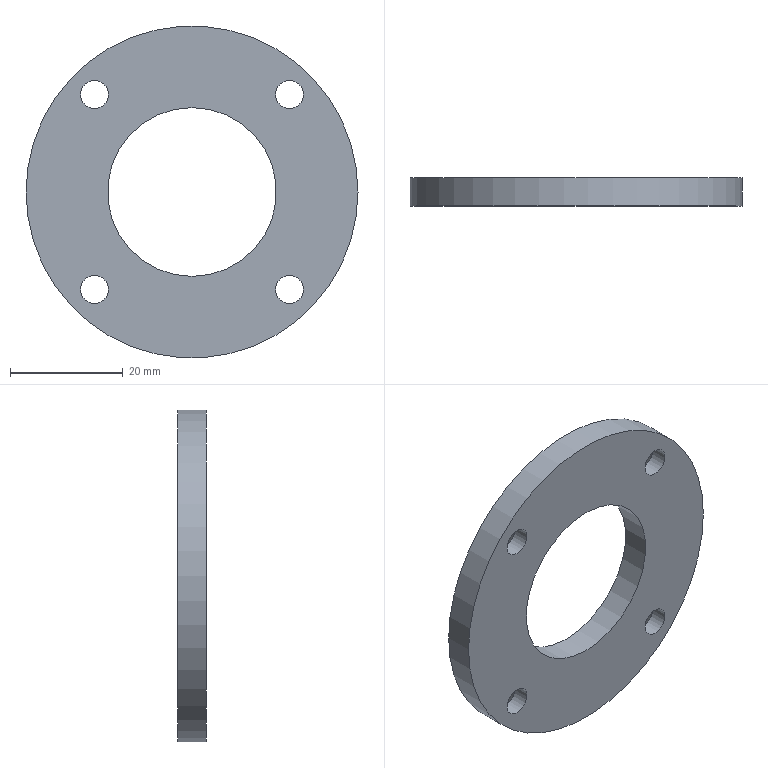Part | STEP file | 冲床-300配套压波_id366_x_t | 1 solid | 12 faces | box 59 x 5 x 59 mm | volume 9584 mm3 | cylinder 6 | cone 4 | plane 2 | commonest cylinder face diameters 5 x4 30 x1 59 x1
STEP:
#1=CARTESIAN_POINT('',(1421.5,98.5,80.083));
#2=VERTEX_POINT('',#1);
#3=CARTESIAN_POINT('',(1392.,98.5,80.083));
#4=DIRECTION('',(0.,1.,0.));
#5=DIRECTION('',(1.,0.,0.));
#6=AXIS2_PLACEMENT_3D('',#3,#4,#5);
#7=CIRCLE('',#6,29.5);
#8=EDGE_CURVE('',#2,#2,#7,.T.);
#9=ORIENTED_EDGE('',*,*,#8,.F.);
#10=EDGE_LOOP('',(#9));
#11=FACE_BOUND('',#10,.T.);
#12=CARTESIAN_POINT('',(1421.5,93.5,80.083));
#13=VERTEX_POINT('',#12);
#14=CARTESIAN_POINT('',(1392.,93.5,80.083));
#15=DIRECTION('',(0.,1.,0.));
#16=DIRECTION('',(1.,0.,0.));
#17=AXIS2_PLACEMENT_3D('',#14,#15,#16);
#18=CIRCLE('',#17,29.5);
#19=EDGE_CURVE('',#13,#13,#18,.T.);
#20=ORIENTED_EDGE('',*,*,#19,.T.);
#21=EDGE_LOOP('',(#20));
#22=FACE_BOUND('',#21,.T.);
#23=CARTESIAN_POINT('',(1392.,93.5,80.083));
#24=DIRECTION('',(0.,1.,0.));
#25=DIRECTION('',(0.,0.,-1.));
#26=AXIS2_PLACEMENT_3D('',#23,#24,#25);
#27=CYLINDRICAL_SURFACE('',#26,29.5);
#28=ADVANCED_FACE('',(#11,#22),#27,.T.);
#29=CARTESIAN_POINT('',(1409.324,93.5,94.908));
#30=VERTEX_POINT('',#29);
#31=CARTESIAN_POINT('',(1409.324,93.5,97.408));
#32=DIRECTION('',(0.,1.,0.));
#33=DIRECTION('',(0.,0.,-1.));
#34=AXIS2_PLACEMENT_3D('',#31,#32,#33);
#35=CIRCLE('',#34,2.5);
#36=EDGE_CURVE('',#30,#30,#35,.T.);
#37=ORIENTED_EDGE('',*,*,#36,.T.);
#38=EDGE_LOOP('',(#37));
#39=FACE_BOUND('',#38,.T.);
#40=CARTESIAN_POINT('',(1374.676,93.5,94.908));
#41=VERTEX_POINT('',#40);
#42=CARTESIAN_POINT('',(1374.676,93.5,97.408));
#43=DIRECTION('',(0.,1.,0.));
#44=DIRECTION('',(0.,0.,-1.));
#45=AXIS2_PLACEMENT_3D('',#42,#43,#44);
#46=CIRCLE('',#45,2.5);
#47=EDGE_CURVE('',#41,#41,#46,.T.);
#48=ORIENTED_EDGE('',*,*,#47,.T.);
#49=EDGE_LOOP('',(#48));
#50=FACE_BOUND('',#49,.T.);
#51=CARTESIAN_POINT('',(1374.676,93.5,60.259));
#52=VERTEX_POINT('',#51);
#53=CARTESIAN_POINT('',(1374.676,93.5,62.759));
#54=DIRECTION('',(0.,1.,0.));
#55=DIRECTION('',(0.,0.,-1.));
#56=AXIS2_PLACEMENT_3D('',#53,#54,#55);
#57=CIRCLE('',#56,2.5);
#58=EDGE_CURVE('',#52,#52,#57,.T.);
#59=ORIENTED_EDGE('',*,*,#58,.T.);
#60=EDGE_LOOP('',(#59));
#61=FACE_BOUND('',#60,.T.);
#62=CARTESIAN_POINT('',(1409.324,93.5,60.259));
#63=VERTEX_POINT('',#62);
#64=CARTESIAN_POINT('',(1409.324,93.5,62.759));
#65=DIRECTION('',(0.,1.,0.));
#66=DIRECTION('',(0.,0.,-1.));
#67=AXIS2_PLACEMENT_3D('',#64,#65,#66);
#68=CIRCLE('',#67,2.5);
#69=EDGE_CURVE('',#63,#63,#68,.T.);
#70=ORIENTED_EDGE('',*,*,#69,.T.);
#71=EDGE_LOOP('',(#70));
#72=FACE_BOUND('',#71,.T.);
#73=CARTESIAN_POINT('',(1392.,93.5,65.083));
#74=VERTEX_POINT('',#73);
#75=CARTESIAN_POINT('',(1392.,93.5,80.083));
#76=DIRECTION('',(0.,1.,0.));
#77=DIRECTION('',(0.,0.,-1.));
#78=AXIS2_PLACEMENT_3D('',#75,#76,#77);
#79=CIRCLE('',#78,15.);
#80=EDGE_CURVE('',#74,#74,#79,.T.);
#81=ORIENTED_EDGE('',*,*,#80,.T.);
#82=EDGE_LOOP('',(#81));
#83=FACE_BOUND('',#82,.T.);
#84=ORIENTED_EDGE('',*,*,#19,.F.);
#85=EDGE_LOOP('',(#84));
#86=FACE_BOUND('',#85,.T.);
#87=CARTESIAN_POINT('',(1392.,93.5,80.083));
#88=DIRECTION('',(0.,1.,0.));
#89=DIRECTION('',(0.,0.,-1.));
#90=AXIS2_PLACEMENT_3D('',#87,#88,#89);
#91=PLANE('',#90);
#92=ADVANCED_FACE('',(#39,#50,#61,#72,#83,#86),#91,.F.);
#93=CARTESIAN_POINT('',(1374.676,98.5,58.259));
#94=VERTEX_POINT('',#93);
#95=CARTESIAN_POINT('',(1374.676,98.5,62.759));
#96=DIRECTION('',(0.,-1.,0.));
#97=DIRECTION('',(0.,0.,-1.));
#98=AXIS2_PLACEMENT_3D('',#95,#96,#97);
#99=CIRCLE('',#98,4.5);
#100=EDGE_CURVE('',#94,#94,#99,.T.);
#101=ORIENTED_EDGE('',*,*,#100,.T.);
#102=EDGE_LOOP('',(#101));
#103=FACE_BOUND('',#102,.T.);
#104=CARTESIAN_POINT('',(1409.324,98.5,58.259));
#105=VERTEX_POINT('',#104);
#106=CARTESIAN_POINT('',(1409.324,98.5,62.759));
#107=DIRECTION('',(0.,-1.,0.));
#108=DIRECTION('',(0.,0.,-1.));
#109=AXIS2_PLACEMENT_3D('',#106,#107,#108);
#110=CIRCLE('',#109,4.5);
#111=EDGE_CURVE('',#105,#105,#110,.T.);
#112=ORIENTED_EDGE('',*,*,#111,.T.);
#113=EDGE_LOOP('',(#112));
#114=FACE_BOUND('',#113,.T.);
#115=CARTESIAN_POINT('',(1409.324,98.5,92.908));
#116=VERTEX_POINT('',#115);
#117=CARTESIAN_POINT('',(1409.324,98.5,97.408));
#118=DIRECTION('',(0.,-1.,0.));
#119=DIRECTION('',(0.,0.,-1.));
#120=AXIS2_PLACEMENT_3D('',#117,#118,#119);
#121=CIRCLE('',#120,4.5);
#122=EDGE_CURVE('',#116,#116,#121,.T.);
#123=ORIENTED_EDGE('',*,*,#122,.T.);
#124=EDGE_LOOP('',(#123));
#125=FACE_BOUND('',#124,.T.);
#126=CARTESIAN_POINT('',(1374.676,98.5,92.908));
#127=VERTEX_POINT('',#126);
#128=CARTESIAN_POINT('',(1374.676,98.5,97.408));
#129=DIRECTION('',(0.,-1.,0.));
#130=DIRECTION('',(0.,0.,-1.));
#131=AXIS2_PLACEMENT_3D('',#128,#129,#130);
#132=CIRCLE('',#131,4.5);
#133=EDGE_CURVE('',#127,#127,#132,.T.);
#134=ORIENTED_EDGE('',*,*,#133,.T.);
#135=EDGE_LOOP('',(#134));
#136=FACE_BOUND('',#135,.T.);
#137=CARTESIAN_POINT('',(1392.,98.5,65.083));
#138=VERTEX_POINT('',#137);
#139=CARTESIAN_POINT('',(1392.,98.5,80.083));
#140=DIRECTION('',(0.,1.,0.));
#141=DIRECTION('',(0.,0.,-1.));
#142=AXIS2_PLACEMENT_3D('',#139,#140,#141);
#143=CIRCLE('',#142,15.);
#144=EDGE_CURVE('',#138,#138,#143,.T.);
#145=ORIENTED_EDGE('',*,*,#144,.F.);
#146=EDGE_LOOP('',(#145));
#147=FACE_BOUND('',#146,.T.);
#148=ORIENTED_EDGE('',*,*,#8,.T.);
#149=EDGE_LOOP('',(#148));
#150=FACE_BOUND('',#149,.T.);
#151=CARTESIAN_POINT('',(1392.,98.5,80.083));
#152=DIRECTION('',(0.,1.,0.));
#153=DIRECTION('',(0.,0.,-1.));
#154=AXIS2_PLACEMENT_3D('',#151,#152,#153);
#155=PLANE('',#154);
#156=ADVANCED_FACE('',(#103,#114,#125,#136,#147,#150),#155,.T.);
#157=ORIENTED_EDGE('',*,*,#144,.T.);
#158=EDGE_LOOP('',(#157));
#159=FACE_BOUND('',#158,.T.);
#160=ORIENTED_EDGE('',*,*,#80,.F.);
#161=EDGE_LOOP('',(#160));
#162=FACE_BOUND('',#161,.T.);
#163=CARTESIAN_POINT('',(1392.,69.5,80.083));
#164=DIRECTION('',(0.,1.,0.));
#165=DIRECTION('',(1.,0.,0.));
#166=AXIS2_PLACEMENT_3D('',#163,#164,#165);
#167=CYLINDRICAL_SURFACE('',#166,15.);
#168=ADVANCED_FACE('',(#159,#162),#167,.F.);
#169=CARTESIAN_POINT('',(1409.324,96.5,60.259));
#170=VERTEX_POINT('',#169);
#171=CARTESIAN_POINT('',(1409.324,96.5,62.759));
#172=DIRECTION('',(0.,1.,0.));
#173=DIRECTION('',(0.,0.,-1.));
#174=AXIS2_PLACEMENT_3D('',#171,#172,#173);
#175=CIRCLE('',#174,2.5);
#176=EDGE_CURVE('',#170,#170,#175,.T.);
#177=ORIENTED_EDGE('',*,*,#176,.T.);
#178=EDGE_LOOP('',(#177));
#179=FACE_BOUND('',#178,.T.);
#180=ORIENTED_EDGE('',*,*,#69,.F.);
#181=EDGE_LOOP('',(#180));
#182=FACE_BOUND('',#181,.T.);
#183=CARTESIAN_POINT('',(1409.324,59.5,62.759));
#184=DIRECTION('',(0.,1.,0.));
#185=DIRECTION('',(0.,0.,-1.));
#186=AXIS2_PLACEMENT_3D('',#183,#184,#185);
#187=CYLINDRICAL_SURFACE('',#186,2.5);
#188=ADVANCED_FACE('',(#179,#182),#187,.F.);
#189=CARTESIAN_POINT('',(1374.676,96.5,60.259));
#190=VERTEX_POINT('',#189);
#191=CARTESIAN_POINT('',(1374.676,96.5,62.759));
#192=DIRECTION('',(0.,1.,0.));
#193=DIRECTION('',(0.,0.,-1.));
#194=AXIS2_PLACEMENT_3D('',#191,#192,#193);
#195=CIRCLE('',#194,2.5);
#196=EDGE_CURVE('',#190,#190,#195,.T.);
#197=ORIENTED_EDGE('',*,*,#196,.T.);
#198=EDGE_LOOP('',(#197));
#199=FACE_BOUND('',#198,.T.);
#200=ORIENTED_EDGE('',*,*,#58,.F.);
#201=EDGE_LOOP('',(#200));
#202=FACE_BOUND('',#201,.T.);
#203=CARTESIAN_POINT('',(1374.676,59.5,62.759));
#204=DIRECTION('',(0.,1.,0.));
#205=DIRECTION('',(0.,0.,-1.));
#206=AXIS2_PLACEMENT_3D('',#203,#204,#205);
#207=CYLINDRICAL_SURFACE('',#206,2.5);
#208=ADVANCED_FACE('',(#199,#202),#207,.F.);
#209=CARTESIAN_POINT('',(1374.676,96.5,94.908));
#210=VERTEX_POINT('',#209);
#211=CARTESIAN_POINT('',(1374.676,96.5,97.408));
#212=DIRECTION('',(0.,1.,0.));
#213=DIRECTION('',(0.,0.,-1.));
#214=AXIS2_PLACEMENT_3D('',#211,#212,#213);
#215=CIRCLE('',#214,2.5);
#216=EDGE_CURVE('',#210,#210,#215,.T.);
#217=ORIENTED_EDGE('',*,*,#216,.T.);
#218=EDGE_LOOP('',(#217));
#219=FACE_BOUND('',#218,.T.);
#220=ORIENTED_EDGE('',*,*,#47,.F.);
#221=EDGE_LOOP('',(#220));
#222=FACE_BOUND('',#221,.T.);
#223=CARTESIAN_POINT('',(1374.676,59.5,97.408));
#224=DIRECTION('',(0.,1.,0.));
#225=DIRECTION('',(0.,0.,-1.));
#226=AXIS2_PLACEMENT_3D('',#223,#224,#225);
#227=CYLINDRICAL_SURFACE('',#226,2.5);
#228=ADVANCED_FACE('',(#219,#222),#227,.F.);
#229=CARTESIAN_POINT('',(1409.324,96.5,94.908));
#230=VERTEX_POINT('',#229);
#231=CARTESIAN_POINT('',(1409.324,96.5,97.408));
#232=DIRECTION('',(0.,1.,0.));
#233=DIRECTION('',(0.,0.,-1.));
#234=AXIS2_PLACEMENT_3D('',#231,#232,#233);
#235=CIRCLE('',#234,2.5);
#236=EDGE_CURVE('',#230,#230,#235,.T.);
#237=ORIENTED_EDGE('',*,*,#236,.T.);
#238=EDGE_LOOP('',(#237));
#239=FACE_BOUND('',#238,.T.);
#240=ORIENTED_EDGE('',*,*,#36,.F.);
#241=EDGE_LOOP('',(#240));
#242=FACE_BOUND('',#241,.T.);
#243=CARTESIAN_POINT('',(1409.324,59.5,97.408));
#244=DIRECTION('',(0.,1.,0.));
#245=DIRECTION('',(0.,0.,-1.));
#246=AXIS2_PLACEMENT_3D('',#243,#244,#245);
#247=CYLINDRICAL_SURFACE('',#246,2.5);
#248=ADVANCED_FACE('',(#239,#242),#247,.F.);
#249=ORIENTED_EDGE('',*,*,#100,.F.);
#250=EDGE_LOOP('',(#249));
#251=FACE_BOUND('',#250,.T.);
#252=ORIENTED_EDGE('',*,*,#196,.F.);
#253=EDGE_LOOP('',(#252));
#254=FACE_BOUND('',#253,.T.);
#255=CARTESIAN_POINT('',(1374.676,96.5,62.759));
#256=DIRECTION('',(0.,1.,0.));
#257=DIRECTION('',(0.,0.,-1.));
#258=AXIS2_PLACEMENT_3D('',#255,#256,#257);
#259=CONICAL_SURFACE('',#258,2.5,45.);
#260=ADVANCED_FACE('',(#251,#254),#259,.F.);
#261=ORIENTED_EDGE('',*,*,#111,.F.);
#262=EDGE_LOOP('',(#261));
#263=FACE_BOUND('',#262,.T.);
#264=ORIENTED_EDGE('',*,*,#176,.F.);
#265=EDGE_LOOP('',(#264));
#266=FACE_BOUND('',#265,.T.);
#267=CARTESIAN_POINT('',(1409.324,96.5,62.759));
#268=DIRECTION('',(0.,1.,0.));
#269=DIRECTION('',(0.,0.,-1.));
#270=AXIS2_PLACEMENT_3D('',#267,#268,#269);
#271=CONICAL_SURFACE('',#270,2.5,45.);
#272=ADVANCED_FACE('',(#263,#266),#271,.F.);
#273=ORIENTED_EDGE('',*,*,#122,.F.);
#274=EDGE_LOOP('',(#273));
#275=FACE_BOUND('',#274,.T.);
#276=ORIENTED_EDGE('',*,*,#236,.F.);
#277=EDGE_LOOP('',(#276));
#278=FACE_BOUND('',#277,.T.);
#279=CARTESIAN_POINT('',(1409.324,96.5,97.408));
#280=DIRECTION('',(0.,1.,0.));
#281=DIRECTION('',(0.,0.,-1.));
#282=AXIS2_PLACEMENT_3D('',#279,#280,#281);
#283=CONICAL_SURFACE('',#282,2.5,45.);
#284=ADVANCED_FACE('',(#275,#278),#283,.F.);
#285=ORIENTED_EDGE('',*,*,#133,.F.);
#286=EDGE_LOOP('',(#285));
#287=FACE_BOUND('',#286,.T.);
#288=ORIENTED_EDGE('',*,*,#216,.F.);
#289=EDGE_LOOP('',(#288));
#290=FACE_BOUND('',#289,.T.);
#291=CARTESIAN_POINT('',(1374.676,96.5,97.408));
#292=DIRECTION('',(0.,1.,0.));
#293=DIRECTION('',(0.,0.,-1.));
#294=AXIS2_PLACEMENT_3D('',#291,#292,#293);
#295=CONICAL_SURFACE('',#294,2.5,45.);
#296=ADVANCED_FACE('',(#287,#290),#295,.F.);
#297=CLOSED_SHELL('',(#28,#92,#156,#168,#188,#208,#228,#248,#260,#272,#284,#296));
#298=MANIFOLD_SOLID_BREP('',#297);
#299=(LENGTH_UNIT()NAMED_UNIT(*)SI_UNIT(.MILLI.,.METRE.));
#300=UNCERTAINTY_MEASURE_WITH_UNIT(LENGTH_MEASURE(0.00002),#299,'','');
#301=(NAMED_UNIT(*)PLANE_ANGLE_UNIT()SI_UNIT($,.RADIAN.));
#302=PLANE_ANGLE_MEASURE_WITH_UNIT(PLANE_ANGLE_MEASURE(0.01745),#301);
#303=DIMENSIONAL_EXPONENTS(0.,0.,0.,0.,0.,0.,0.);
#304=(CONVERSION_BASED_UNIT('DEGREE',#302)NAMED_UNIT(#303)PLANE_ANGLE_UNIT());
#305=(NAMED_UNIT(*)SI_UNIT($,.STERADIAN.)SOLID_ANGLE_UNIT());
#306=(GEOMETRIC_REPRESENTATION_CONTEXT(3)GLOBAL_UNCERTAINTY_ASSIGNED_CONTEXT((#300))GLOBAL_UNIT_ASSIGNED_CONTEXT((#299,#304,#305))REPRESENTATION_CONTEXT('',''));
#307=ADVANCED_BREP_SHAPE_REPRESENTATION('',(#298),#306);